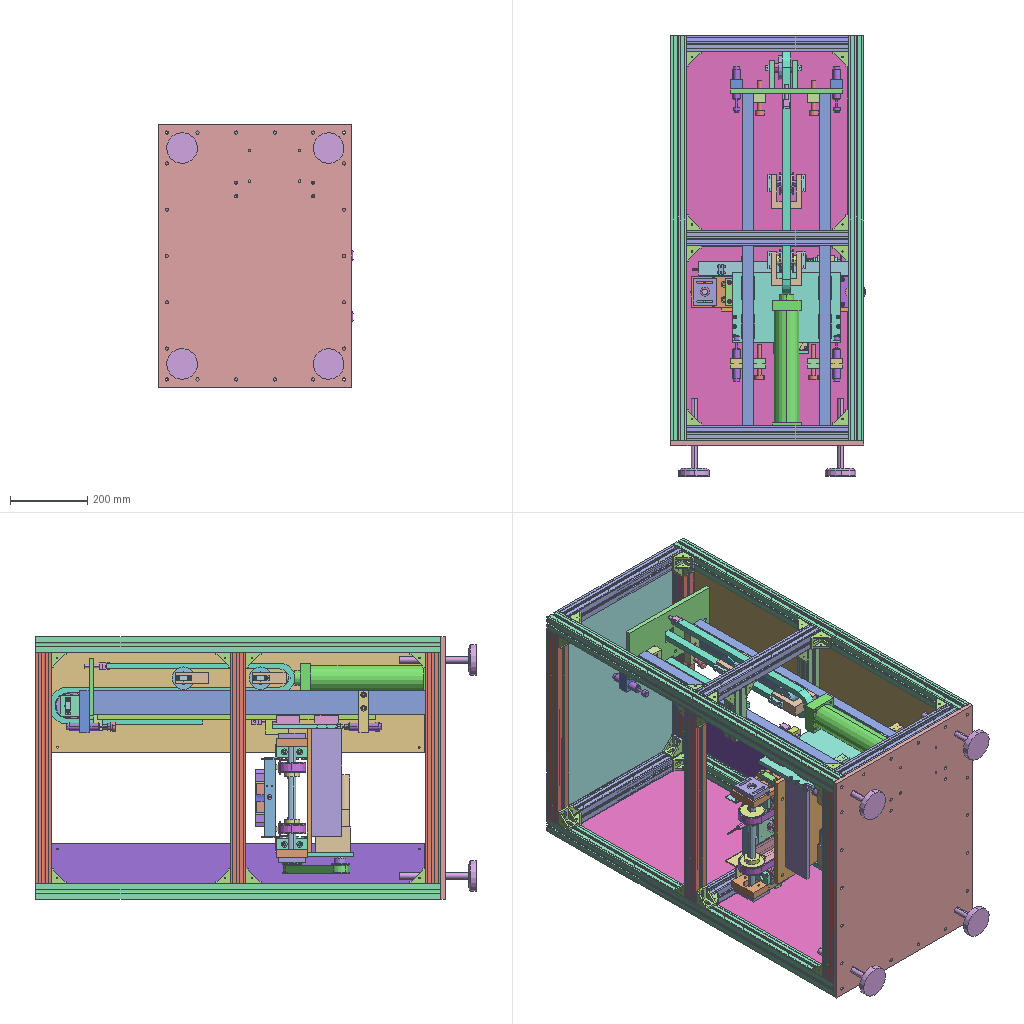Assembly | STEP file | 76 different items | 186 placed | box 503 x 1142 x 680 mm
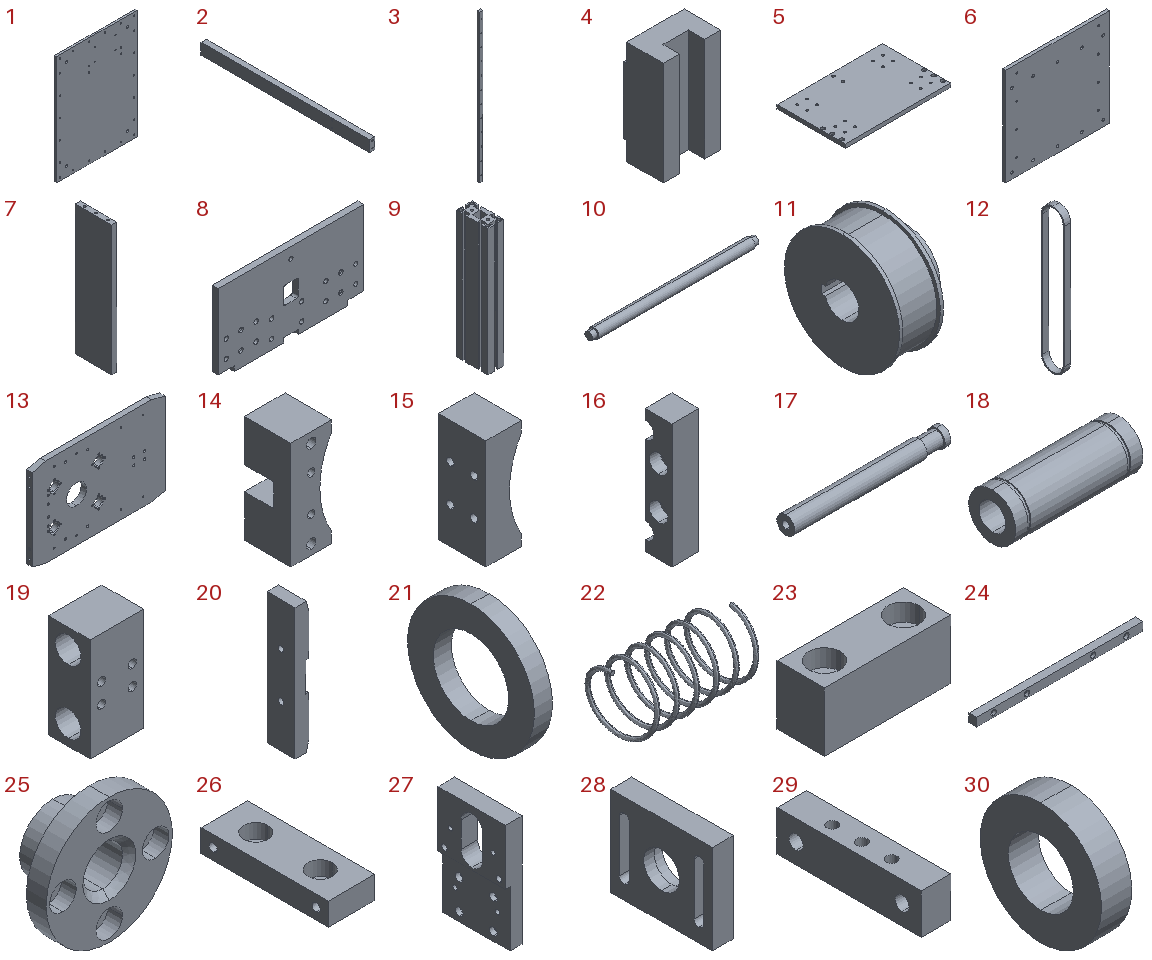Parts list (item | name | quantity | parent item | size | volume):
1 | PA-8-6(base plate) | x1 | - | 500 x 12 x 680 mm | 4053163 mm3
2 | PA-7-7(guide rail mounting plate) | x2 | in PA-8(guide rail assembly) | 28 x 900 x 60 mm | 1504828 mm3
3 | PA-7-9(HGH15CA guide rail) | x2 | in PA-8(guide rail assembly) | 15 x 14 x 720 mm | 146714 mm3
4 | PA-7-8(HGH15CA slider) | x4 | in PA-8(guide rail assembly) | 34 x 23.7 x 61.4 mm | 38690 mm3
5 | PA-7-10(connecting block) | x1 | in PA-8(guide rail assembly) | 280 x 180 x 10 mm | 491440 mm3
6 | PA-7-11 (support block) | x1 | in PA-8(guide rail assembly) | 340 x 10 x 320 mm | 1077927 mm3
7 | PA-7-12(inclined block) | x2 | in PA-8(guide rail assembly) | 11 x 79 x 280 mm | 242077 mm3
8 | PA-7-13(fixed block) | x1 | in PA-8(guide rail assembly) | 292 x 12 x 160 mm | 521488 mm3
9 | PA-7-27(cross beam) | x2 | in PA-8(conveyor assembly) | 40 x 80 x 320 mm | 588947 mm3
10 | PA-7-36(secondary shaft) | x1 | in PA-8(conveyor assembly) | 328 x 20 x 20 mm | 99023 mm3
11 | PA-7-37(wheel) | x4 | in PA-8(conveyor assembly) | 38 x 68 x 68 mm | 87974 mm3
12 | PA-7-38(conveyor belt) | x2 | in PA-8(conveyor assembly) | 20 x 72 x 452 mm | 77890 mm3
13 | PA-3-1(tooling plate) | x1 | in PA-3(tooling assembly, return) | 300 x 12 x 200 mm | 673943 mm3
14 | PA-3-4(semicircular tube block) | x1 | in PA-3(tooling assembly, return) | 28 x 32 x 74 mm | 45440 mm3
15 | PA-3-5(movable semicircular tube block) | x1 | in PA-3(spring pressure assembly) | 24 x 32 x 74 mm | 45434 mm3
16 | PA-3-7(clamp block) | x2 | in PA-3(spring pressure assembly) | 16 x 16 x 74 mm | 15676 mm3
17 | PA-3-6(guide rod) | x2 | in PA-3(spring pressure assembly) | 105 x 12 x 12 mm | 11156 mm3
18 | PA-3-9(linear bearing LM12LUU) | x2 | in PA-3(spring pressure assembly) | 57 x 21 x 21 mm | 13212 mm3
19 | PA-3-8(guide bushing seat) | x1 | in PA-3(spring pressure assembly) | 43.4 x 34 x 84 mm | 87676 mm3
20 | PA-3-10(connecting plate) | x1 | in PA-3(spring pressure assembly) | 16 x 32 x 150 mm | 73689 mm3
21 | PA-3-11(stop plate) | x2 | in PA-3(spring pressure assembly) | 3 x 21 x 21 mm | 670.926 mm3
22 | PA-3-12(spring) | x2 | in PA-3(spring pressure assembly) | 31 x 16 x 16 mm | 222.275 mm3
23 | PA-3-13(elastic rubber) | x2 | in PA-3(tooling assembly, return) | 32 x 12 x 15 mm | 4980 mm3
24 | PA-3-17(guide strip) | x2 | in PA-3(tooling assembly, return) | 250 x 12 x 12.5 mm | 36132 mm3
25 | PA-3-18(guide bushing) | x4 | in PA-3(tooling assembly, return) | 38 x 17 x 38 mm | 7268 mm3
26 | PA-7-39(reinforcing block) | x4 | in PA-8(conveyor assembly) | 29 x 79 x 14 mm | 27118 mm3
27 | PA-7-35(connecting plate) | x2 | in PA-7(secondary end seat assembly) | 19.5 x 79 x 130 mm | 136895 mm3
28 | PA-7-28(secondary shaft seat) | x2 | in PA-7(secondary end seat assembly) | 14 x 68 x 60 mm | 42344 mm3
29 | PA-7-29(fixed plate) | x2 | in PA-7(secondary end seat assembly) | 14 x 68 x 19 mm | 15184 mm3
30 | PA-7-30(ZZ6902) | x2 | in PA-7(secondary end seat assembly) | 7 x 28 x 28 mm | 3073 mm3
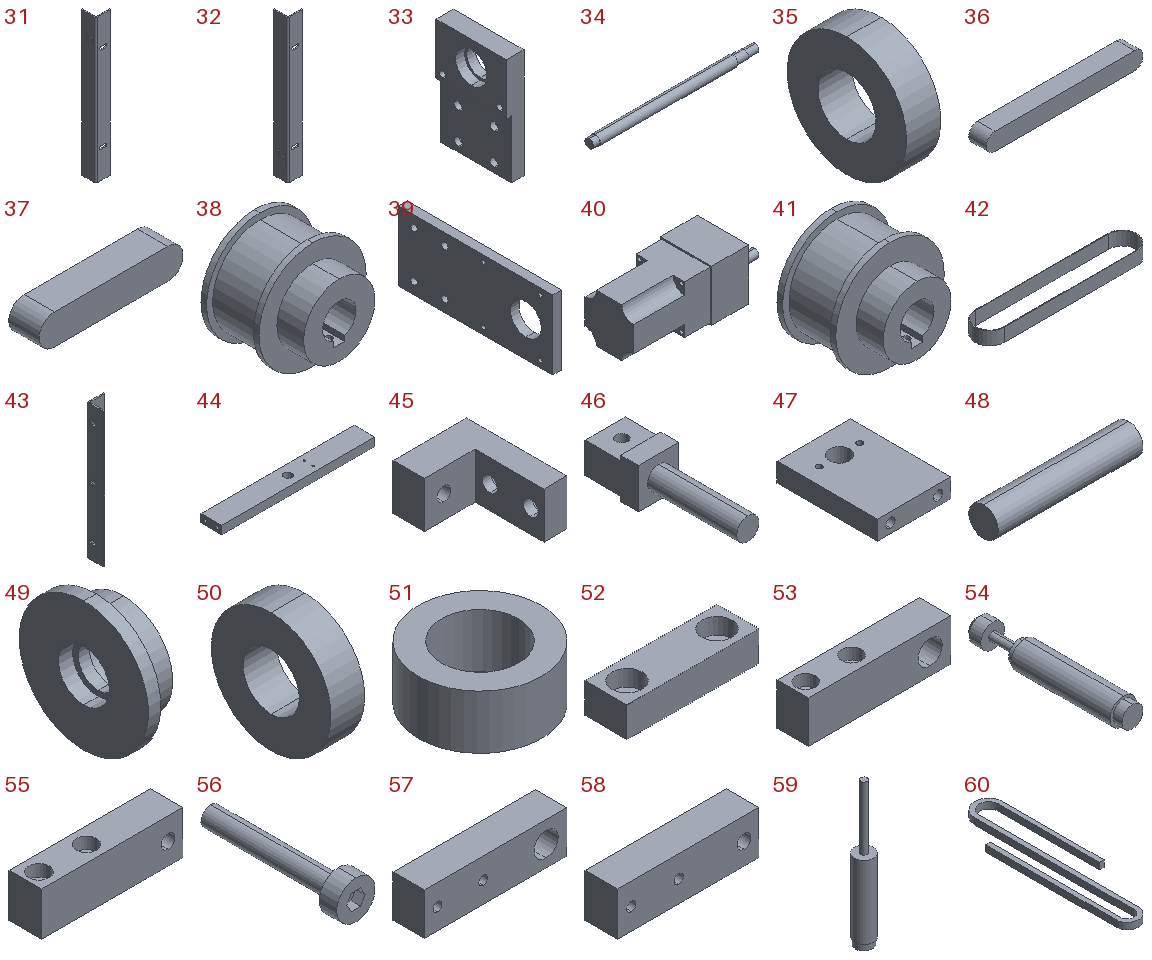31 | PA-7-40A(edge stop plate) | x1 | in PA-8(conveyor assembly) | 40 x 40 x 400 mm | 89658 mm3
32 | PA-7-40B(edge stop plate) | x1 | in PA-8(conveyor assembly) | 40 x 40 x 400 mm | 89658 mm3
33 | PA-7-41(connecting plate) | x2 | in PA-8(conveyor assembly) | 19.5 x 79 x 122 mm | 133748 mm3
34 | PA-7-43(main shaft) | x1 | in PA-8(conveyor assembly) | 325 x 20 x 20 mm | 94666 mm3
35 | PA-7-42(ZZ6003) | x2 | in PA-8(conveyor assembly) | 10 x 35 x 35 mm | 7351 mm3
36 | PA-7-44(5x5x40 key) | x4 | in PA-8(conveyor assembly) | 45 x 5 x 5 mm | 1098 mm3
37 | PA-7-45(4x4x15 key) | x1 | in PA-8(conveyor assembly) | 19 x 4 x 4 mm | 290.265 mm3
38 | PA-7-33(ATP14L075)_ATP22XL050-A-H8 | x1 | in PA-8(conveyor assembly) | 48 x 38 x 48 mm | 41242 mm3
39 | PA-7-34(motor mounting plate) | x1 | in PA-7(motor assembly) | 11 x 200 x 90 mm | 180816 mm3
40 | PA-7-32(60W.1: 15) | x1 | in PA-7(motor assembly) | 238 x 90 x 90 mm | 1379919 mm3
41 | PA-7-31(ATP14L075)_ATP22XL050-A-H8 | x1 | in PA-7(motor assembly) | 48 x 38 x 48 mm | 40082 mm3
42 | PA-7-46(timing belt 210L,width 20,Z=56) | x1 | in PA-8(conveyor assembly) | 244.45 x 44.45 x 20 mm | 10730 mm3
43 | PA-7-57(belt support block) | x2 | in PA-8(conveyor assembly) | 40 x 40 x 340 mm | 77417 mm3
44 | PA-7-72(stop block) | x1 | in PA-8(conveyor assembly) | 206 x 28 x 11 mm | 61677 mm3
45 | PA-7-48(connecting block) | x1 | in PA-8(guide rail assembly) | 45 x 61 x 28 mm | 35599 mm3
46 | PA-7-47(hook) | x2 | in PA-8(guide rail assembly) | 18 x 64 x 18 mm | 9415 mm3
47 | PA-7-49(support block) | x2 | in PA-7(transfer wheel assembly) | 54 x 74 x 14 mm | 51598 mm3
48 | PA-7-23(shaft rod) | x1 | in PA-7(transfer wheel assembly) | 74 x 15 x 15 mm | 13077 mm3
49 | PA-7-21(z=16,p=15.875 sprocket) | x1 | in PA-7(sprocket) | 25 x 81.37 x 81.37 mm | 74577 mm3
50 | PA-7-24(ZZ6002) | x4 | in PA-7(sprocket), PA-7(sprocket assembly) | 9 x 32 x 32 mm | 5648 mm3
51 | PA-7-50(stop plate) | x2 | in PA-7(transfer wheel assembly) | 24 x 24 x 10.5 mm | 2895 mm3
52 | PA-7-51(stop block) | x6 | in PA-7(transfer wheel assembly), PA-7(sprocket assembly) | 44 x 14 x 10 mm | 5093 mm3
53 | PA-7-68(buffer fixing block) | x2 | in PA-7(lower buffer assembly) | 109 x 24 x 32 mm | 69208 mm3
54 | PA-7-70(hydraulic buffer ACA2020) | x4 | in PA-7(lower buffer assembly), PA-7(upper buffer assembly) | 20 x 118 x 20 mm | 29167 mm3
55 | PA-7-69(positioning block) | x2 | in PA-7(lower positioning assembly) | 104 x 24 x 32 mm | 69858 mm3
56 | PA-7-71(M12X60) | x4 | in PA-7(lower positioning assembly), PA-7(upper positioning assembly) | 24 x 91 x 24 mm | 13504 mm3
57 | PA-7-68A(buffer fixing block) | x2 | in PA-7(upper buffer assembly) | 109 x 24 x 32 mm | 75518 mm3
58 | PA-7-69A(positioning block) | x2 | in PA-7(upper positioning assembly) | 104 x 24 x 32 mm | 76168 mm3
59 | PA-8-5(M12-4 proximity switch) | x1 | in PA-8(guide rail assembly) | 12 x 12 x 90 mm | 6055 mm3
60 | PA-7-54(chain) | x1 | - | 158.46 x 636.775 x 22 mm | 522937 mm3
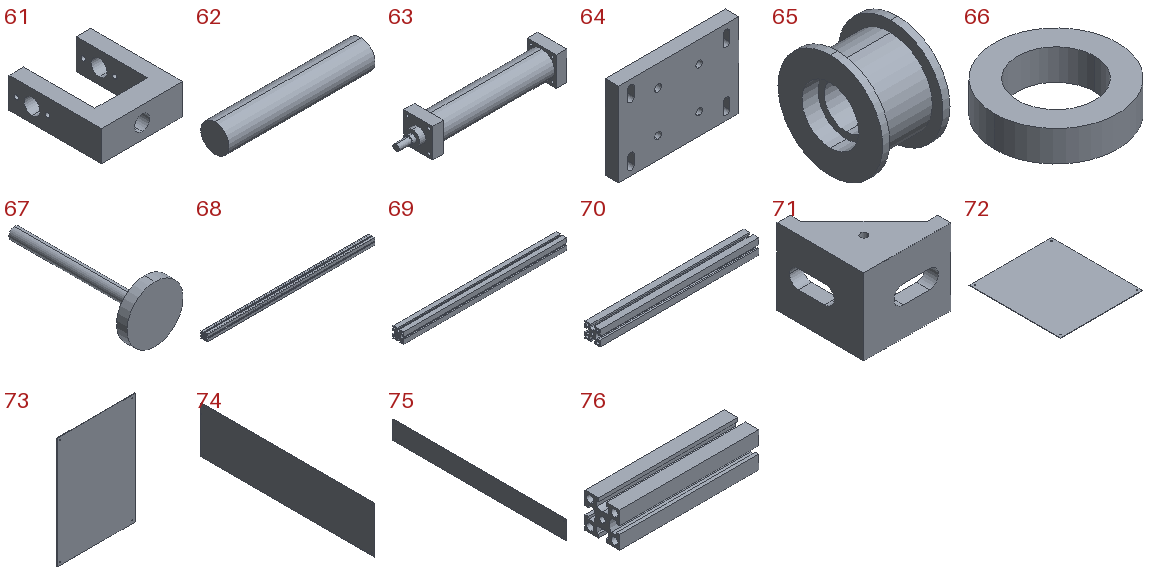61 | PA-7-22(connecting block) | x2 | in PA-7(sprocket assembly) | 78 x 88 x 29 mm | 91430 mm3
62 | PA-7-55(shaft rod) | x2 | in PA-7(sprocket assembly) | 78 x 15 x 15 mm | 13784 mm3
63 | PA-7-15(SC63X250) | x1 | in PA-7(sprocket assembly) | 403 x 75 x 75 mm | 1293600 mm3
64 | PA-7-25(fixed plate) | x1 | in PA-7(sprocket assembly) | 164 x 18 x 114 mm | 315701 mm3
65 | PA-7-52(pulley) | x2 | in PA-7(sprocket assembly) | 38 x 59 x 59 mm | 49626 mm3
66 | PA-7-53(stop plate) | x2 | in PA-7(sprocket assembly) | 24 x 24 x 6 mm | 1654 mm3
67 | PA-1-6(M16x200 foot cup) | x4 | - | 80 x 200 x 80 mm | 130963 mm3
68 | PA-7-58(vertical stop) | x4 | in PA-8(frame) | 1050 x 40 x 40 mm | 867444 mm3
69 | PA-7-59(cross bar) | x5 | in PA-8(frame) | 600 x 40 x 40 mm | 495706 mm3
70 | PA-7-60(cross bar) | x6 | in PA-8(frame) | 420 x 40 x 40 mm | 346994 mm3
71 | PA-7-61(4040A foot bracket) | x35 | in PA-8(frame) | 40 x 40 x 35 mm | 17755 mm3
72 | PA-7-62(cover plate) | x2 | in PA-8(frame) | 418 x 463 x 2 mm | 386911 mm3
73 | PA-7-64(cover plate) | x1 | in PA-8(frame) | 418 x 2 x 598 mm | 499771 mm3
74 | PA-7-65(cover plate) | x1 | in PA-8(frame) | 2 x 968 x 260 mm | 503203 mm3
75 | PA-7-66(cover plate) | x1 | in PA-8(frame) | 2 x 968 x 104 mm | 201187 mm3
76 | PA-7-67(reinforcing stop) | x2 | - | 160 x 40 x 40 mm | 131462 mm3
Placements (level | parent | child | x y z in mm | rotation matrix by rows):
1 | subassembly 2 | PA-8-6(base plate) | 231.231 -175.56 350.0 | 1 0 0 0 1 0 0 0 1
1 | subassembly 2 | PA-8(guide rail assembly) | 237.273 41.493 180.0 | 1 0 0 0 1 0 0 0 1
2 | PA-8(guide rail assembly) | PA-7-7(guide rail mounting plate) | -56.042 -205.053 -30.0 | 1 0 0 0 1 0 0 0 1
2 | PA-8(guide rail assembly) | PA-7-9(HGH15CA guide rail) | -56.042 684.947 -30.0 | 1 0 0 0 0 1 0 -1 0
2 | PA-8(guide rail assembly) | PA-7-8(HGH15CA slider) | -56.042 90.647 -34.3 | 1 0 0 0 0 1 0 -1 -0
2 | PA-8(guide rail assembly) | PA-7-7(guide rail mounting plate) | 143.958 -205.053 -30.0 | 1 0 0 0 1 0 0 0 1
2 | PA-8(guide rail assembly) | PA-7-9(HGH15CA guide rail) | 143.958 684.947 -30.0 | 1 0 0 0 0 1 0 -1 0
2 | PA-8(guide rail assembly) | PA-7-8(HGH15CA slider) | 143.958 90.647 -34.3 | 1 0 0 0 0 1 0 -1 -0
2 | PA-8(guide rail assembly) | PA-7-10(connecting block) | 43.958 140.647 -68.0 | 1 0 0 0 1 0 0 0 1
2 | PA-8(guide rail assembly) | PA-7-11 (support block) | 43.958 130.647 -68.0 | 1 0 0 0 1 0 0 0 1
2 | PA-8(guide rail assembly) | PA-7-12(inclined block) | 177.958 51.647 -68.0 | 1 0 0 0 1 0 0 0 1
2 | PA-8(guide rail assembly) | PA-7-12(inclined block) | -90.042 51.647 -68.0 | 1 0 0 0 1 0 0 0 1
2 | PA-8(guide rail assembly) | PA-7-13(fixed block) | 43.958 694.947 -45.0 | 1 0 0 0 1 0 0 0 1
2 | PA-8(guide rail assembly) | PA-8(conveyor assembly) | -18.042 169.332 -81.67 | 0 0 -1 0 1 0 1 0 -0
3 | PA-8(conveyor assembly) | PA-7-27(cross beam) | -46.33 11.315 -200.0 | 1 0 0 0 1 0 0 0 1
3 | PA-8(conveyor assembly) | PA-7-27(cross beam) | -286.33 11.315 -200.0 | 1 0 0 0 1 0 0 0 1
3 | PA-8(conveyor assembly) | PA-7-36(secondary shaft) | -330.33 11.315 150.0 | 1 0 0 0 0.9618 -0.2738 0 0.2738 0.9618
3 | PA-8(conveyor assembly) | PA-7-37(wheel) | -73.33 11.315 150.0 | -1 0 0 0 0.9618 0.2738 0 0.2738 -0.9618
3 | PA-8(conveyor assembly) | PA-7-38(conveyor belt) | -86.33 11.315 150.0 | -1 0 0 0 -1 0 0 0 1
3 | PA-8(conveyor assembly) | PA-7-37(wheel) | -259.33 11.315 150.0 | 1 0 0 0 0.9618 -0.2738 0 0.2738 0.9618
3 | PA-8(conveyor assembly) | PA-7-38(conveyor belt) | -246.33 11.315 150.0 | -1 0 0 0 -1 0 0 0 1
3 | PA-8(conveyor assembly) | PA-3(tooling assembly, return) | -166.33 74.53 -98.044 | 0 0 1 0 1 0 -1 0 -0
4 | PA-3(tooling assembly, return) | PA-3-1(tooling plate) | -75.335 -9.216 -0.0 | 1 0 0 0 1 0 0 0 1
4 | PA-3(tooling assembly, return) | PA-3-4(semicircular tube block) | -153.335 12.784 -0.0 | 1 0 0 0 1 0 0 0 1
4 | PA-3(tooling assembly, return) | PA-3(spring pressure assembly) | -58.515 11.875 -0.0 | -1 0 0 0 1 0 0 0 -1
5 | PA-3(spring pressure assembly) | PA-3-5(movable semicircular tube block) | -57.18 2.909 -0.0 | 1 0 0 0 1 0 0 0 1
5 | PA-3(spring pressure assembly) | PA-3-7(clamp block) | -73.18 -13.091 -0.0 | 1 0 0 0 1 0 0 0 1
5 | PA-3(spring pressure assembly) | PA-3-7(clamp block) | -73.18 18.909 -0.0 | 1 0 0 0 -1 0 0 0 -1
5 | PA-3(spring pressure assembly) | PA-3-6(guide rod) | -162.18 2.909 -26.0 | 1 0 0 0 0.9992 -0.03879 0 0.03879 0.9992
5 | PA-3(spring pressure assembly) | PA-3-6(guide rod) | -162.18 2.909 26.0 | 1 0 0 0 0.4218 -0.9067 0 0.9067 0.4218
5 | PA-3(spring pressure assembly) | PA-3-9(linear bearing LM12LUU) | -153.18 2.909 -26.0 | 1 0 0 0 1 0 0 0 1
5 | PA-3(spring pressure assembly) | PA-3-9(linear bearing LM12LUU) | -153.18 2.909 26.0 | 1 0 0 0 1 0 0 0 1
5 | PA-3(spring pressure assembly) | PA-3-8(guide bushing seat) | -124.68 -15.091 -0.0 | 1 0 0 0 1 0 0 0 1
5 | PA-3(spring pressure assembly) | PA-3-10(connecting plate) | -178.18 2.909 -0.0 | 1 0 0 0 1 0 0 0 1
5 | PA-3(spring pressure assembly) | PA-3-11(stop plate) | -96.18 2.909 26.0 | 1 0 0 0 1 0 0 0 1
5 | PA-3(spring pressure assembly) | PA-3-11(stop plate) | -96.18 2.909 -26.0 | 1 0 0 0 1 0 0 0 1
5 | PA-3(spring pressure assembly) | PA-3-12(spring) | -97.732 2.909 26.0 | 1 0 0 0 1 0 0 0 1
5 | PA-3(spring pressure assembly) | PA-3-12(spring) | -97.081 2.909 -26.0 | 1 0 0 0 0.9742 -0.2257 0 0.2257 0.9742
4 | PA-3(tooling assembly, return) | PA-3-13(elastic rubber) | -175.335 -9.216 -70.0 | 0 0 -1 0 1 0 1 0 0
4 | PA-3(tooling assembly, return) | PA-3-13(elastic rubber) | -175.335 -9.216 70.0 | 0 0 -1 0 1 0 1 0 0
4 | PA-3(tooling assembly, return) | PA-3-17(guide strip) | -25.335 -27.215 80.0 | 1 0 0 0 1 0 0 0 1
4 | PA-3(tooling assembly, return) | PA-3-17(guide strip) | -25.335 -27.215 -80.0 | 1 0 0 0 1 0 0 0 1
4 | PA-3(tooling assembly, return) | PA-3-18(guide bushing) | -125.335 -21.215 40.0 | 1 0 0 0 1 0 0 0 1
4 | PA-3(tooling assembly, return) | PA-3-18(guide bushing) | -125.335 -21.215 -40.0 | 1 0 0 0 1 0 0 0 1
4 | PA-3(tooling assembly, return) | PA-3-18(guide bushing) | -25.335 -21.215 40.0 | 1 0 0 0 1 0 0 0 1
4 | PA-3(tooling assembly, return) | PA-3-18(guide bushing) | -25.335 -21.215 -40.0 | 1 0 0 0 1 0 0 0 1
3 | PA-8(conveyor assembly) | PA-7-39(reinforcing block) | -46.33 11.315 120.0 | 1 0 0 0 1 0 0 0 1
3 | PA-8(conveyor assembly) | PA-7-39(reinforcing block) | -286.33 11.315 120.0 | 1 0 0 0 1 0 0 0 1
3 | PA-8(conveyor assembly) | PA-7-39(reinforcing block) | -46.33 11.315 -200.0 | -1 0 0 0 1 0 0 0 -1
3 | PA-8(conveyor assembly) | PA-7-39(reinforcing block) | -286.33 11.315 -200.0 | -1 0 0 0 1 0 0 0 -1
3 | PA-8(conveyor assembly) | PA-7(secondary end seat assembly) | -332.66 22.63 -80.0 | -1 0 0 0 -1 0 0 0 1
4 | PA-7(secondary end seat assembly) | PA-7-35(connecting plate) | -31.83 11.315 135.0 | 1 0 0 0 1 0 0 0 1
4 | PA-7(secondary end seat assembly) | PA-7-28(secondary shaft seat) | -5.33 11.315 230.0 | -1 0 0 0 1 0 0 0 -1
4 | PA-7(secondary end seat assembly) | PA-7-29(fixed plate) | -5.33 11.315 167.0 | 1 0 0 0 1 0 0 0 1
4 | PA-7(secondary end seat assembly) | PA-7-30(ZZ6902) | -12.33 11.315 230.0 | 1 0 0 0 1 0 0 0 1
3 | PA-8(conveyor assembly) | PA-7(secondary end seat assembly) | -0.0 0.0 -80.0 | 1 0 0 0 1 0 0 0 1
4 | PA-7(secondary end seat assembly) | PA-7-35(connecting plate) | -31.83 11.315 135.0 | 1 0 0 0 1 0 0 0 1
4 | PA-7(secondary end seat assembly) | PA-7-28(secondary shaft seat) | -5.33 11.315 230.0 | -1 0 0 0 1 0 0 0 -1
4 | PA-7(secondary end seat assembly) | PA-7-29(fixed plate) | -5.33 11.315 167.0 | 1 0 0 0 1 0 0 0 1
4 | PA-7(secondary end seat assembly) | PA-7-30(ZZ6902) | -12.33 11.315 230.0 | 1 0 0 0 1 0 0 0 1
3 | PA-8(conveyor assembly) | PA-7-40A(edge stop plate) | -66.33 51.315 167.248 | 1 0 0 0 1 0 0 0 1
3 | PA-8(conveyor assembly) | PA-7-40B(edge stop plate) | -266.33 51.315 -233.53 | -1 0 0 0 1 0 0 0 -1
3 | PA-8(conveyor assembly) | PA-7-41(connecting plate) | -31.83 11.315 -135.0 | 1 0 0 0 -1 0 0 0 -1
3 | PA-8(conveyor assembly) | PA-7-41(connecting plate) | -300.83 11.315 -135.0 | -1 0 0 0 1 0 0 0 -1
3 | PA-8(conveyor assembly) | PA-7-43(main shaft) | -19.83 11.315 -230.0 | -1 0 0 0 0.9997 0.02567 0 0.02567 -0.9997
3 | PA-8(conveyor assembly) | PA-7-42(ZZ6003) | -310.83 11.315 -230.0 | 1 0 0 0 1 0 0 0 1
3 | PA-8(conveyor assembly) | PA-7-42(ZZ6003) | -31.83 11.315 -230.0 | 1 0 0 0 1 0 0 0 1
3 | PA-8(conveyor assembly) | PA-7-44(5x5x40 key) | -240.33 18.047 151.917 | 1 0 0 0 0.9618 -0.2738 0 0.2738 0.9618
3 | PA-8(conveyor assembly) | PA-7-44(5x5x40 key) | -92.33 18.047 151.917 | 1 0 0 0 0.9618 -0.2738 0 0.2738 0.9618
3 | PA-8(conveyor assembly) | PA-7-44(5x5x40 key) | -240.33 18.313 -229.82 | 1 0 0 0 0.9997 -0.02567 0 0.02567 0.9997
3 | PA-8(conveyor assembly) | PA-7-44(5x5x40 key) | -92.33 18.313 -229.82 | 1 0 0 0 0.9997 -0.02567 0 0.02567 0.9997
3 | PA-8(conveyor assembly) | PA-7-37(wheel) | -73.33 11.315 -230.0 | -1 0 0 0 0.9997 0.02567 0 0.02567 -0.9997
3 | PA-8(conveyor assembly) | PA-7-37(wheel) | -259.33 11.315 -230.0 | 1 0 0 0 0.9997 -0.02567 0 0.02567 0.9997
3 | PA-8(conveyor assembly) | PA-7-45(4x4x15 key) | -333.33 16.313 -229.872 | 1 0 0 0 0.9997 -0.02567 0 0.02567 0.9997
3 | PA-8(conveyor assembly) | PA-7-33(ATP14L075)_ATP22XL050-A-H8 | -337.33 11.315 -230.0 | 0 -1 0 0.9317 0 -0.3631 0.3631 0 0.9317
3 | PA-8(conveyor assembly) | PA-7(motor assembly) | -349.597 -58.379 -73.875 | -1 0 0 0 1 0 0 0 -1
4 | PA-7(motor assembly) | PA-7-34(motor mounting plate) | -37.767 -90.306 -0.0 | 1 0 0 0 1 0 0 0 1
4 | PA-7(motor assembly) | PA-7-32(60W.1: 15) | -108.267 -37.306 -0.0 | 1 0 0 0 1 0 0 0 1
4 | PA-7(motor assembly) | PA-7-31(ATP14L075)_ATP22XL050-A-H8 | -12.267 -55.306 -0.0 | 0 1 0 -0.1427 0 -0.9898 -0.9898 0 0.1427
3 | PA-8(conveyor assembly) | PA-7-46(timing belt 210L,width 20,Z=56) | -351.58 -51.185 -151.938 | 0 0 1 0.625 0.7806 0 -0.7806 0.625 0
3 | PA-8(conveyor assembly) | PA-7-57(belt support block) | -266.33 3.315 130.0 | 1 0 0 0 1 0 0 0 1
3 | PA-8(conveyor assembly) | PA-7-57(belt support block) | -66.33 3.315 -210.0 | -1 0 0 0 1 0 0 0 -1
3 | PA-8(conveyor assembly) | PA-7-72(stop block) | -163.33 55.315 108.089 | 1 0 0 0 1 0 0 0 1
2 | PA-8(guide rail assembly) | PA-7-8(HGH15CA slider) | -56.042 190.647 -34.3 | 1 0 0 0 0 1 0 -1 -0
2 | PA-8(guide rail assembly) | PA-7-8(HGH15CA slider) | 143.958 190.647 -34.3 | 1 0 0 0 0 1 0 -1 -0
2 | PA-8(guide rail assembly) | PA-7-48(connecting block) | 43.958 188.647 -82.0 | 0 0 1 0 1 0 -1 0 0
2 | PA-8(guide rail assembly) | PA-7-47(hook) | 43.958 220.647 -49.0 | 0 0 1 0 1 0 -1 0 0
2 | PA-8(guide rail assembly) | PA-7(transfer wheel assembly) | 5.358 752.51 1.624 | 0 0 -1 0 1 0 1 0 0
3 | PA-7(transfer wheel assembly) | PA-7-49(support block) | -9.939 -45.563 -0.0 | 1 0 0 0 1 0 0 0 1
3 | PA-7(transfer wheel assembly) | PA-7-49(support block) | -9.939 -45.563 -60.0 | 1 0 0 0 1 0 0 0 1
3 | PA-7(transfer wheel assembly) | PA-7-23(shaft rod) | -9.939 9.437 -30.0 | 0 -0.03289 0.9995 0 0.9995 0.03289 -1 0 0
3 | PA-7(transfer wheel assembly) | PA-7(sprocket) | -9.323 17.636 -38.04 | 0 0.07491 -0.9972 0 0.9972 0.07491 1 0 0
4 | PA-7(sprocket) | PA-7-21(z=16,p=15.875 sprocket) | -4.46 -8.221 0.0 | 1 0 0 0 0.8869 -0.4619 0 0.4619 0.8869
4 | PA-7(sprocket) | PA-7-24(ZZ6002) | 11.54 -8.221 0.0 | 1 0 0 0 1 0 0 0 1
4 | PA-7(sprocket) | PA-7-24(ZZ6002) | -4.46 -8.221 0.0 | 1 0 0 0 1 0 0 0 1
3 | PA-7(transfer wheel assembly) | PA-7-50(stop plate) | -9.939 9.437 -17.5 | 1 0 0 0 1 0 0 0 1
3 | PA-7(transfer wheel assembly) | PA-7-50(stop plate) | -9.939 9.437 -53.0 | 0.9993 0.03637 0 -0.03637 0.9993 0 0 0 1
3 | PA-7(transfer wheel assembly) | PA-7-51(stop block) | -9.939 9.437 7.0 | 1 0 0 0 1 0 0 0 1
3 | PA-7(transfer wheel assembly) | PA-7-51(stop block) | -9.939 9.437 -67.0 | -1 0 0 0 1 0 0 0 -1
2 | PA-8(guide rail assembly) | PA-7-47(hook) | 43.958 718.947 93.5 | 0 0 -1 0 -1 0 -1 0 0
2 | PA-8(guide rail assembly) | PA-7(lower buffer assembly) | 173.958 -10.863 -72.058 | 0 0 1 0 1 0 -1 0 0
3 | PA-7(lower buffer assembly) | PA-7-68(buffer fixing block) | -102.058 5.81 -0.0 | 1 0 0 0 1 0 0 0 1
3 | PA-7(lower buffer assembly) | PA-7-70(hydraulic buffer ACA2020) | -9.058 -40.34 -0.0 | 1 0 0 0 1 0 0 0 1
2 | PA-8(guide rail assembly) | PA-7(lower buffer assembly) | -86.042 -10.863 -72.058 | 0 0 1 0 1 0 -1 0 0
3 | PA-7(lower buffer assembly) | PA-7-68(buffer fixing block) | -102.058 5.81 -0.0 | 1 0 0 0 1 0 0 0 1
3 | PA-7(lower buffer assembly) | PA-7-70(hydraulic buffer ACA2020) | -9.058 -40.34 -0.0 | 1 0 0 0 1 0 0 0 1
2 | PA-8(guide rail assembly) | PA-7(lower positioning assembly) | -26.042 -3.218 -34.749 | 0 0 -1 0 -1 0 -1 0 0
3 | PA-7(lower positioning assembly) | PA-7-69(positioning block) | -64.749 1.835 -0.0 | 1 0 0 0 1 0 0 0 1
3 | PA-7(lower positioning assembly) | PA-7-71(M12X60) | 28.251 43.274 0.0 | -0.9457 0 0.3251 0 -1 0 0.3251 0 0.9457
2 | PA-8(guide rail assembly) | PA-7(lower positioning assembly) | 113.958 -3.218 -34.749 | 0 0 -1 0 -1 0 -1 0 0
3 | PA-7(lower positioning assembly) | PA-7-69(positioning block) | -64.749 1.835 -0.0 | 1 0 0 0 1 0 0 0 1
3 | PA-7(lower positioning assembly) | PA-7-71(M12X60) | 28.251 43.274 0.0 | -0.9457 0 0.3251 0 -1 0 0.3251 0 0.9457
2 | PA-8(guide rail assembly) | PA-7(upper buffer assembly) | 173.958 724.757 -72.058 | 0 0 -1 0 -1 0 -1 0 -0
3 | PA-7(upper buffer assembly) | PA-7-68A(buffer fixing block) | -102.058 5.81 -0.0 | 1 0 0 0 1 0 0 0 1
3 | PA-7(upper buffer assembly) | PA-7-70(hydraulic buffer ACA2020) | -9.058 -40.34 -0.0 | 1 0 0 0 1 0 0 0 1
2 | PA-8(guide rail assembly) | PA-7(upper buffer assembly) | -86.042 724.757 -72.058 | 0 0 -1 0 -1 0 -1 0 -0
3 | PA-7(upper buffer assembly) | PA-7-68A(buffer fixing block) | -102.058 5.81 -0.0 | 1 0 0 0 1 0 0 0 1
3 | PA-7(upper buffer assembly) | PA-7-70(hydraulic buffer ACA2020) | -9.058 -40.34 -0.0 | 1 0 0 0 1 0 0 0 1
2 | PA-8(guide rail assembly) | PA-7(upper positioning assembly) | 113.958 681.112 -34.749 | 0 0 1 0 1 0 -1 0 -0
3 | PA-7(upper positioning assembly) | PA-7-69A(positioning block) | -64.749 1.835 -0.0 | 1 0 0 0 1 0 0 0 1
3 | PA-7(upper positioning assembly) | PA-7-71(M12X60) | 28.251 -42.058 0.0 | 0.9854 0 0.1701 0 1 0 -0.1701 0 0.9854
2 | PA-8(guide rail assembly) | PA-7(upper positioning assembly) | -26.042 681.112 -34.749 | 0 0 1 0 1 0 -1 0 -0
3 | PA-7(upper positioning assembly) | PA-7-69A(positioning block) | -64.749 1.835 -0.0 | 1 0 0 0 1 0 0 0 1
3 | PA-7(upper positioning assembly) | PA-7-71(M12X60) | 28.251 -42.058 0.0 | 0.9854 0 0.1701 0 1 0 -0.1701 0 0.9854
2 | PA-8(guide rail assembly) | PA-8-5(M12-4 proximity switch) | -109.856 238.647 -245.0 | 0 0 -1 -0.3449 0.9386 0 0.9386 0.3449 -0
1 | subassembly 2 | PA-7-54(chain) | 281.231 103.441 171.685 | 0 0 1 0 1 0 -1 0 0
1 | subassembly 2 | PA-7(sprocket assembly) | 331.761 295.662 243.0 | 1 0 0 0 1 0 0 0 1
2 | PA-7(sprocket assembly) | PA-7-22(connecting block) | -50.53 -58.221 -0.0 | 1 0 0 0 1 0 0 0 1
2 | PA-7(sprocket assembly) | PA-7-55(shaft rod) | -50.53 7.779 0.0 | 1 0 0 0 -0.9998 -0.01988 0 0.01988 -0.9998
2 | PA-7(sprocket assembly) | PA-7-15(SC63X250) | -50.53 -413.721 -0.0 | 0 1 0 -1 0 0 0 0 1
2 | PA-7(sprocket assembly) | PA-7-25(fixed plate) | -50.53 -450.221 -0.0 | 1 0 0 0 1 0 0 0 1
2 | PA-7(sprocket assembly) | PA-7-51(stop block) | -89.53 7.779 -0.0 | 0 0 -1 -1 0 0 0 1 0
2 | PA-7(sprocket assembly) | PA-7-51(stop block) | -11.53 7.779 0.0 | 0 0 1 -1 0 0 0 -1 0
2 | PA-7(sprocket assembly) | PA-7-52(pulley) | -69.53 7.779 0.0 | 1 0 0 0 0.9396 -0.3422 0 0.3422 0.9396
2 | PA-7(sprocket assembly) | PA-7-24(ZZ6002) | -40.53 7.779 -0.0 | 1 0 0 0 1 0 0 0 1
2 | PA-7(sprocket assembly) | PA-7-24(ZZ6002) | -69.53 7.779 -0.0 | 1 0 0 0 1 0 0 0 1
2 | PA-7(sprocket assembly) | PA-7-53(stop plate) | -25.53 7.779 -0.0 | 0 0 -1 0 1 0 1 0 0
2 | PA-7(sprocket assembly) | PA-7-53(stop plate) | -69.53 7.779 -0.0 | 0 0 -1 0.4887 0.8725 0 0.8725 -0.4887 0
2 | PA-7(sprocket assembly) | PA-7-55(shaft rod) | -50.53 207.779 -0.0 | 1 0 0 0 -0.9998 -0.01988 0 0.01988 -0.9998
2 | PA-7(sprocket assembly) | PA-7-51(stop block) | -89.53 207.779 -0.0 | 0 0 -1 -1 0 0 0 1 0
2 | PA-7(sprocket assembly) | PA-7-51(stop block) | -11.53 207.779 0.0 | 0 0 1 -1 0 0 0 -1 0
2 | PA-7(sprocket assembly) | PA-7-22(connecting block) | -50.53 141.779 -0.0 | 1 0 0 0 1 0 0 0 1
2 | PA-7(sprocket assembly) | PA-7-52(pulley) | -69.53 207.779 0.0 | 1 0 0 0 0.9396 -0.3422 0 0.3422 0.9396
1 | subassembly 2 | PA-1-6(M16x200 foot cup) | 421.231 -255.56 290.0 | 0.9984 0 0.05706 0 1 0 -0.05706 0 0.9984
1 | subassembly 2 | PA-1-6(M16x200 foot cup) | 41.231 -255.56 290.0 | 0.9984 0 0.05706 0 1 0 -0.05706 0 0.9984
1 | subassembly 2 | PA-1-6(M16x200 foot cup) | 421.231 -255.56 -270.0 | 0.9984 0 0.05706 0 1 0 -0.05706 0 0.9984
1 | subassembly 2 | PA-1-6(M16x200 foot cup) | 41.231 -255.56 -270.0 | 0.9984 0 0.05706 0 1 0 -0.05706 0 0.9984
1 | subassembly 2 | PA-8(frame) | 0.0 190.0 -0.0 | 1 0 0 0 1 0 0 0 1
2 | PA-8(frame) | PA-7-58(vertical stop) | 461.231 696.441 330.0 | 0 1 0 -1 0 0 0 0 1
2 | PA-8(frame) | PA-7-58(vertical stop) | 461.231 696.441 -310.0 | 0 1 0 -1 0 0 0 0 1
2 | PA-8(frame) | PA-7-58(vertical stop) | 1.231 696.441 -310.0 | 0 1 0 -1 0 0 0 0 1
2 | PA-8(frame) | PA-7-58(vertical stop) | 1.231 696.441 330.0 | 0 1 0 -1 0 0 0 0 1
2 | PA-8(frame) | PA-7-59(cross bar) | 461.231 676.441 310.0 | 0 0 1 0 1 0 -1 0 0
2 | PA-8(frame) | PA-7-59(cross bar) | 1.231 676.441 310.0 | 0 0 1 0 1 0 -1 0 0
2 | PA-8(frame) | PA-7-60(cross bar) | 21.231 676.441 -310.0 | 1 0 0 0 1 0 0 0 1
2 | PA-8(frame) | PA-7-60(cross bar) | 21.231 676.441 330.0 | 1 0 0 0 1 0 0 0 1
2 | PA-8(frame) | PA-7-60(cross bar) | 21.231 -333.56 -310.0 | 1 0 0 0 1 0 0 0 1
2 | PA-8(frame) | PA-7-59(cross bar) | 461.231 -333.56 310.0 | 0 0 1 0 1 0 -1 0 0
2 | PA-8(frame) | PA-7-59(cross bar) | 1.231 -333.56 310.0 | 0 0 1 0 1 0 -1 0 0
2 | PA-8(frame) | PA-7-60(cross bar) | 21.231 -333.56 330.0 | 1 0 0 0 1 0 0 0 1
2 | PA-8(frame) | PA-7-61(4040A foot bracket) | 461.231 -313.56 -290.0 | 0 0 -1 0 1 0 1 0 -0
2 | PA-8(frame) | PA-7-61(4040A foot bracket) | 461.231 -313.56 310.0 | 0 0 1 0 1 0 -1 0 0
2 | PA-8(frame) | PA-7-61(4040A foot bracket) | 461.231 656.441 310.0 | 0 0 -1 0 -1 0 -1 0 0
2 | PA-8(frame) | PA-7-61(4040A foot bracket) | 461.231 656.441 -290.0 | 0 0 1 0 -1 0 1 0 0
2 | PA-8(frame) | PA-7-61(4040A foot bracket) | 1.231 656.441 -290.0 | 0 0 1 0 -1 0 1 0 0
2 | PA-8(frame) | PA-7-61(4040A foot bracket) | 1.231 -313.56 -290.0 | 0 0 1 1 0 0 0 1 0
2 | PA-8(frame) | PA-7-61(4040A foot bracket) | 1.231 -313.56 310.0 | 0 0 -1 1 0 0 0 -1 -0
2 | PA-8(frame) | PA-7-61(4040A foot bracket) | 1.231 656.441 310.0 | 0 0 -1 0 -1 0 -1 0 -0
2 | PA-8(frame) | PA-7-61(4040A foot bracket) | 21.231 -313.56 330.0 | 0 1 0 1 0 0 0 0 -1
2 | PA-8(frame) | PA-7-61(4040A foot bracket) | 441.231 -313.56 330.0 | 0 -1 0 1 0 0 0 0 1
2 | PA-8(frame) | PA-7-61(4040A foot bracket) | 441.231 656.441 330.0 | -1 0 0 0 -1 0 0 0 1
2 | PA-8(frame) | PA-7-61(4040A foot bracket) | 21.231 656.441 330.0 | 1 0 0 0 -1 0 0 0 -1
2 | PA-8(frame) | PA-7-61(4040A foot bracket) | 21.231 656.441 -310.0 | 1 0 0 0 -1 0 0 0 -1
2 | PA-8(frame) | PA-7-61(4040A foot bracket) | 21.231 -313.56 -310.0 | 0 1 0 1 0 0 0 0 -1
2 | PA-8(frame) | PA-7-61(4040A foot bracket) | 441.231 -313.56 -310.0 | -1 0 0 0 1 0 0 0 -1
2 | PA-8(frame) | PA-7-61(4040A foot bracket) | 441.231 656.441 -310.0 | 0 -1 0 -1 0 0 0 0 -1
2 | PA-8(frame) | PA-7-59(cross bar) | 1.231 171.44 310.0 | 0 0 1 0 1 0 -1 0 0
2 | PA-8(frame) | PA-7-60(cross bar) | 21.231 171.44 330.0 | 1 0 0 0 1 0 0 0 1
2 | PA-8(frame) | PA-7-60(cross bar) | 21.231 171.44 -310.0 | 1 0 0 0 1 0 0 0 1
2 | PA-8(frame) | PA-7-61(4040A foot bracket) | 1.231 151.44 -290.0 | 0 0 -1 -1 0 0 0 1 -0
2 | PA-8(frame) | PA-7-61(4040A foot bracket) | 1.231 151.44 310.0 | 0 0 -1 0 -1 0 -1 0 -0
2 | PA-8(frame) | PA-7-61(4040A foot bracket) | 1.231 191.44 310.0 | 0 0 1 0 1 0 -1 0 0
2 | PA-8(frame) | PA-7-61(4040A foot bracket) | 1.231 191.44 -290.0 | 0 0 -1 0 1 0 1 0 -0
2 | PA-8(frame) | PA-7-61(4040A foot bracket) | 441.231 191.44 330.0 | 0 -1 0 1 0 0 0 0 1
2 | PA-8(frame) | PA-7-61(4040A foot bracket) | 21.231 191.44 330.0 | 0 1 0 1 0 0 0 0 -1
2 | PA-8(frame) | PA-7-61(4040A foot bracket) | 21.231 151.44 330.0 | 1 0 0 0 -1 0 0 0 -1
2 | PA-8(frame) | PA-7-61(4040A foot bracket) | 441.231 151.44 330.0 | -1 0 0 0 -1 0 0 0 1
2 | PA-8(frame) | PA-7-61(4040A foot bracket) | 21.231 191.44 -310.0 | 0 1 0 1 0 0 0 0 -1
2 | PA-8(frame) | PA-7-61(4040A foot bracket) | 441.231 191.44 -310.0 | -1 0 0 0 1 0 0 0 -1
2 | PA-8(frame) | PA-7-61(4040A foot bracket) | 21.231 151.44 -310.0 | 1 0 0 0 -1 0 0 0 -1
2 | PA-8(frame) | PA-7-61(4040A foot bracket) | 441.231 151.44 -310.0 | 0 -1 0 -1 0 0 0 0 -1
2 | PA-8(frame) | PA-7-62(cover plate) | 231.231 423.94 -327.5 | 1 0 0 0 1 0 0 0 1
2 | PA-8(frame) | PA-7-62(cover plate) | 231.231 -81.059 -327.5 | 1 0 0 0 1 0 0 0 1
2 | PA-8(frame) | PA-7-61(4040A foot bracket) | 21.231 676.441 -290.0 | 1 0 0 0 0 -1 0 1 -0
2 | PA-8(frame) | PA-7-61(4040A foot bracket) | 441.231 676.441 -290.0 | 0 -1 0 0 0 -1 1 0 -0
2 | PA-8(frame) | PA-7-61(4040A foot bracket) | 441.231 676.441 310.0 | -1 0 0 0 0 -1 0 -1 0
2 | PA-8(frame) | PA-7-61(4040A foot bracket) | 21.231 676.441 310.0 | 0 1 0 0 0 -1 -1 0 0
2 | PA-8(frame) | PA-7-64(cover plate) | 231.231 695.941 10.0 | 1 0 0 0 1 0 0 0 1
2 | PA-8(frame) | PA-7-65(cover plate) | 480.731 171.44 179.0 | 1 0 0 0 1 0 0 0 1
2 | PA-8(frame) | PA-7-66(cover plate) | 480.731 171.44 -237.0 | 1 0 0 0 1 0 0 0 1
1 | subassembly 2 | PA-7-67(reinforcing stop) | 415.231 361.44 150.0 | 0 0 -1 0 1 0 1 0 -0
1 | subassembly 2 | PA-7-67(reinforcing stop) | 147.231 361.44 150.0 | 0 0 -1 0 1 0 1 0 -0
1 | subassembly 2 | PA-7-61(4040A foot bracket) | 127.231 361.44 310.0 | 0 -1 0 0 0 1 -1 0 -0
1 | subassembly 2 | PA-7-61(4040A foot bracket) | 167.231 361.44 310.0 | 0 1 0 0 0 -1 -1 0 0
1 | subassembly 2 | PA-7-61(4040A foot bracket) | 395.231 361.44 310.0 | 0 -1 0 0 0 1 -1 0 -0